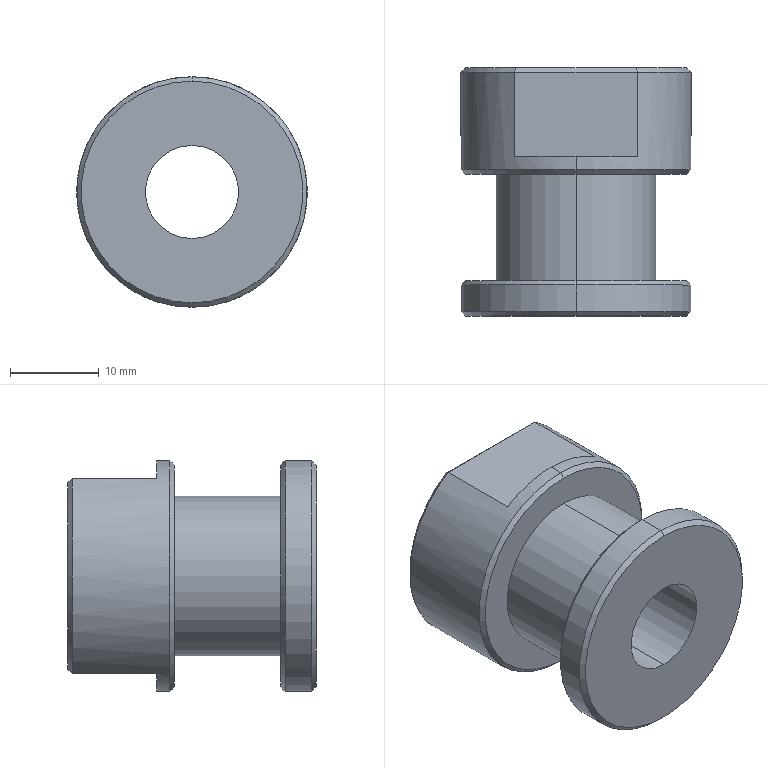Part | STEP file | 03-32SC Floating Joint | 1 solid | 52 faces | box 26 x 28 x 26 mm | volume 2635 mm3 | plane 20 | cone 16 | cylinder 16 | commonest cylinder face diameters 24.84 x4 26 x4 10.5 x2 12.16 x2 16.84 x2 18 x2
STEP:
#1=CARTESIAN_POINT('',(0.,-16.,-12.5));
#2=VERTEX_POINT('',#1);
#3=CARTESIAN_POINT('',(0.,-16.,12.5));
#4=VERTEX_POINT('',#3);
#5=CARTESIAN_POINT('',(0.,-16.,0.));
#6=DIRECTION('',(0.,-1.,0.));
#7=DIRECTION('',(0.,0.,-1.));
#8=AXIS2_PLACEMENT_3D('',#5,#6,#7);
#9=CIRCLE('',#8,12.5);
#10=EDGE_CURVE('',#2,#4,#9,.T.);
#11=ORIENTED_EDGE('',*,*,#10,.F.);
#12=CARTESIAN_POINT('',(0.,-15.5,-13.));
#13=VERTEX_POINT('',#12);
#14=CARTESIAN_POINT('',(0.,-16.,-12.5));
#15=DIRECTION('',(0.,0.7071,-0.7071));
#16=VECTOR('',#15,1000.);
#17=LINE('',#14,#16);
#18=EDGE_CURVE('',#2,#13,#17,.T.);
#19=ORIENTED_EDGE('',*,*,#18,.T.);
#20=CARTESIAN_POINT('',(0.,-15.5,13.));
#21=VERTEX_POINT('',#20);
#22=CARTESIAN_POINT('',(0.,-15.5,0.));
#23=DIRECTION('',(0.,1.,0.));
#24=DIRECTION('',(0.,0.,-1.));
#25=AXIS2_PLACEMENT_3D('',#22,#23,#24);
#26=CIRCLE('',#25,13.);
#27=EDGE_CURVE('',#21,#13,#26,.T.);
#28=ORIENTED_EDGE('',*,*,#27,.F.);
#29=CARTESIAN_POINT('',(0.,-16.,12.5));
#30=DIRECTION('',(0.,0.7071,0.7071));
#31=VECTOR('',#30,1000.);
#32=LINE('',#29,#31);
#33=EDGE_CURVE('',#4,#21,#32,.T.);
#34=ORIENTED_EDGE('',*,*,#33,.F.);
#35=EDGE_LOOP('',(#11,#19,#28,#34));
#36=FACE_OUTER_BOUND('',#35,.T.);
#37=CARTESIAN_POINT('',(0.,-16.,0.));
#38=DIRECTION('',(0.,1.,0.));
#39=DIRECTION('',(0.,0.,1.));
#40=AXIS2_PLACEMENT_3D('',#37,#38,#39);
#41=CONICAL_SURFACE('',#40,12.5,0.7854);
#42=ADVANCED_FACE('',(#36),#41,.T.);
#43=CARTESIAN_POINT('',(0.,0.,-12.5));
#44=VERTEX_POINT('',#43);
#45=CARTESIAN_POINT('',(0.,0.,12.5));
#46=VERTEX_POINT('',#45);
#47=CARTESIAN_POINT('',(0.,0.,0.));
#48=DIRECTION('',(0.,-1.,0.));
#49=DIRECTION('',(0.,0.,-1.));
#50=AXIS2_PLACEMENT_3D('',#47,#48,#49);
#51=CIRCLE('',#50,12.5);
#52=EDGE_CURVE('',#44,#46,#51,.T.);
#53=ORIENTED_EDGE('',*,*,#52,.F.);
#54=CARTESIAN_POINT('',(0.,0.5,-13.));
#55=VERTEX_POINT('',#54);
#56=CARTESIAN_POINT('',(0.,0.,-12.5));
#57=DIRECTION('',(0.,0.7071,-0.7071));
#58=VECTOR('',#57,1000.);
#59=LINE('',#56,#58);
#60=EDGE_CURVE('',#44,#55,#59,.T.);
#61=ORIENTED_EDGE('',*,*,#60,.T.);
#62=CARTESIAN_POINT('',(0.,0.5,13.));
#63=VERTEX_POINT('',#62);
#64=CARTESIAN_POINT('',(0.,0.5,0.));
#65=DIRECTION('',(0.,1.,0.));
#66=DIRECTION('',(0.,0.,-1.));
#67=AXIS2_PLACEMENT_3D('',#64,#65,#66);
#68=CIRCLE('',#67,13.);
#69=EDGE_CURVE('',#63,#55,#68,.T.);
#70=ORIENTED_EDGE('',*,*,#69,.F.);
#71=CARTESIAN_POINT('',(0.,0.,12.5));
#72=DIRECTION('',(0.,0.7071,0.7071));
#73=VECTOR('',#72,1000.);
#74=LINE('',#71,#73);
#75=EDGE_CURVE('',#46,#63,#74,.T.);
#76=ORIENTED_EDGE('',*,*,#75,.F.);
#77=EDGE_LOOP('',(#53,#61,#70,#76));
#78=FACE_OUTER_BOUND('',#77,.T.);
#79=CARTESIAN_POINT('',(0.,0.,0.));
#80=DIRECTION('',(0.,1.,0.));
#81=DIRECTION('',(0.,0.,1.));
#82=AXIS2_PLACEMENT_3D('',#79,#80,#81);
#83=CONICAL_SURFACE('',#82,12.5,0.7854);
#84=ADVANCED_FACE('',(#78),#83,.T.);
#85=CARTESIAN_POINT('',(0.,-12.,12.5));
#86=VERTEX_POINT('',#85);
#87=CARTESIAN_POINT('',(0.,-12.,-12.5));
#88=VERTEX_POINT('',#87);
#89=CARTESIAN_POINT('',(0.,-12.,0.));
#90=DIRECTION('',(0.,1.,0.));
#91=DIRECTION('',(0.,0.,1.));
#92=AXIS2_PLACEMENT_3D('',#89,#90,#91);
#93=CIRCLE('',#92,12.5);
#94=EDGE_CURVE('',#86,#88,#93,.T.);
#95=ORIENTED_EDGE('',*,*,#94,.F.);
#96=CARTESIAN_POINT('',(0.,-12.5,13.));
#97=VERTEX_POINT('',#96);
#98=CARTESIAN_POINT('',(0.,-12.5,13.));
#99=DIRECTION('',(0.,-0.7071,0.7071));
#100=VECTOR('',#99,1000.);
#101=LINE('',#98,#100);
#102=EDGE_CURVE('',#86,#97,#101,.T.);
#103=ORIENTED_EDGE('',*,*,#102,.T.);
#104=CARTESIAN_POINT('',(0.,-12.5,-13.));
#105=VERTEX_POINT('',#104);
#106=CARTESIAN_POINT('',(0.,-12.5,0.));
#107=DIRECTION('',(0.,-1.,0.));
#108=DIRECTION('',(0.,0.,1.));
#109=AXIS2_PLACEMENT_3D('',#106,#107,#108);
#110=CIRCLE('',#109,13.);
#111=EDGE_CURVE('',#105,#97,#110,.T.);
#112=ORIENTED_EDGE('',*,*,#111,.F.);
#113=CARTESIAN_POINT('',(0.,-12.5,-13.));
#114=DIRECTION('',(0.,-0.7071,-0.7071));
#115=VECTOR('',#114,1000.);
#116=LINE('',#113,#115);
#117=EDGE_CURVE('',#88,#105,#116,.T.);
#118=ORIENTED_EDGE('',*,*,#117,.F.);
#119=EDGE_LOOP('',(#95,#103,#112,#118));
#120=FACE_OUTER_BOUND('',#119,.T.);
#121=CARTESIAN_POINT('',(0.,-12.5,0.));
#122=DIRECTION('',(0.,-1.,0.));
#123=DIRECTION('',(0.,0.,-1.));
#124=AXIS2_PLACEMENT_3D('',#121,#122,#123);
#125=CONICAL_SURFACE('',#124,13.,0.7854);
#126=ADVANCED_FACE('',(#120),#125,.T.);
#127=CARTESIAN_POINT('',(0.,12.,-5.25));
#128=VERTEX_POINT('',#127);
#129=CARTESIAN_POINT('',(0.,12.,5.25));
#130=VERTEX_POINT('',#129);
#131=CARTESIAN_POINT('',(0.,12.,0.));
#132=DIRECTION('',(0.,1.,0.));
#133=DIRECTION('',(0.,0.,1.));
#134=AXIS2_PLACEMENT_3D('',#131,#132,#133);
#135=CIRCLE('',#134,5.25);
#136=EDGE_CURVE('',#128,#130,#135,.T.);
#137=ORIENTED_EDGE('',*,*,#136,.T.);
#138=CARTESIAN_POINT('',(0.,-16.,5.25));
#139=VERTEX_POINT('',#138);
#140=CARTESIAN_POINT('',(0.,-16.,5.25));
#141=DIRECTION('',(0.,-1.,0.));
#142=VECTOR('',#141,1000.);
#143=LINE('',#140,#142);
#144=EDGE_CURVE('',#130,#139,#143,.T.);
#145=ORIENTED_EDGE('',*,*,#144,.T.);
#146=CARTESIAN_POINT('',(0.,-16.,-5.25));
#147=VERTEX_POINT('',#146);
#148=CARTESIAN_POINT('',(0.,-16.,0.));
#149=DIRECTION('',(0.,-1.,0.));
#150=DIRECTION('',(0.,0.,-1.));
#151=AXIS2_PLACEMENT_3D('',#148,#149,#150);
#152=CIRCLE('',#151,5.25);
#153=EDGE_CURVE('',#139,#147,#152,.T.);
#154=ORIENTED_EDGE('',*,*,#153,.T.);
#155=CARTESIAN_POINT('',(0.,-16.,-5.25));
#156=DIRECTION('',(0.,-1.,0.));
#157=VECTOR('',#156,1000.);
#158=LINE('',#155,#157);
#159=EDGE_CURVE('',#128,#147,#158,.T.);
#160=ORIENTED_EDGE('',*,*,#159,.F.);
#161=EDGE_LOOP('',(#137,#145,#154,#160));
#162=FACE_OUTER_BOUND('',#161,.T.);
#163=CARTESIAN_POINT('',(0.,-16.,0.));
#164=DIRECTION('',(0.,-1.,0.));
#165=DIRECTION('',(0.,0.,-1.));
#166=AXIS2_PLACEMENT_3D('',#163,#164,#165);
#167=CYLINDRICAL_SURFACE('',#166,5.25);
#168=ADVANCED_FACE('',(#162),#167,.F.);
#169=CARTESIAN_POINT('',(0.,0.,-9.));
#170=VERTEX_POINT('',#169);
#171=CARTESIAN_POINT('',(0.,0.,9.));
#172=VERTEX_POINT('',#171);
#173=CARTESIAN_POINT('',(0.,0.,0.));
#174=DIRECTION('',(0.,-1.,0.));
#175=DIRECTION('',(0.,0.,-1.));
#176=AXIS2_PLACEMENT_3D('',#173,#174,#175);
#177=CIRCLE('',#176,9.);
#178=EDGE_CURVE('',#170,#172,#177,.T.);
#179=ORIENTED_EDGE('',*,*,#178,.T.);
#180=CARTESIAN_POINT('',(0.,-12.,9.));
#181=VERTEX_POINT('',#180);
#182=CARTESIAN_POINT('',(0.,12.,9.));
#183=DIRECTION('',(0.,-1.,0.));
#184=VECTOR('',#183,1000.);
#185=LINE('',#182,#184);
#186=EDGE_CURVE('',#172,#181,#185,.T.);
#187=ORIENTED_EDGE('',*,*,#186,.T.);
#188=CARTESIAN_POINT('',(0.,-12.,-9.));
#189=VERTEX_POINT('',#188);
#190=CARTESIAN_POINT('',(0.,-12.,0.));
#191=DIRECTION('',(0.,-1.,0.));
#192=DIRECTION('',(0.,0.,-1.));
#193=AXIS2_PLACEMENT_3D('',#190,#191,#192);
#194=CIRCLE('',#193,9.);
#195=EDGE_CURVE('',#189,#181,#194,.T.);
#196=ORIENTED_EDGE('',*,*,#195,.F.);
#197=CARTESIAN_POINT('',(0.,12.,-9.));
#198=DIRECTION('',(0.,-1.,0.));
#199=VECTOR('',#198,1000.);
#200=LINE('',#197,#199);
#201=EDGE_CURVE('',#170,#189,#200,.T.);
#202=ORIENTED_EDGE('',*,*,#201,.F.);
#203=EDGE_LOOP('',(#179,#187,#196,#202));
#204=FACE_OUTER_BOUND('',#203,.T.);
#205=CARTESIAN_POINT('',(0.,12.,0.));
#206=DIRECTION('',(0.,-1.,0.));
#207=DIRECTION('',(0.,0.,-1.));
#208=AXIS2_PLACEMENT_3D('',#205,#206,#207);
#209=CYLINDRICAL_SURFACE('',#208,9.);
#210=ADVANCED_FACE('',(#204),#209,.T.);
#211=ORIENTED_EDGE('',*,*,#111,.T.);
#212=CARTESIAN_POINT('',(0.,12.,13.));
#213=DIRECTION('',(0.,-1.,0.));
#214=VECTOR('',#213,1000.);
#215=LINE('',#212,#214);
#216=EDGE_CURVE('',#97,#21,#215,.T.);
#217=ORIENTED_EDGE('',*,*,#216,.T.);
#218=ORIENTED_EDGE('',*,*,#27,.T.);
#219=CARTESIAN_POINT('',(0.,12.,-13.));
#220=DIRECTION('',(0.,-1.,0.));
#221=VECTOR('',#220,1000.);
#222=LINE('',#219,#221);
#223=EDGE_CURVE('',#105,#13,#222,.T.);
#224=ORIENTED_EDGE('',*,*,#223,.F.);
#225=EDGE_LOOP('',(#211,#217,#218,#224));
#226=FACE_OUTER_BOUND('',#225,.T.);
#227=CARTESIAN_POINT('',(0.,12.,0.));
#228=DIRECTION('',(0.,-1.,0.));
#229=DIRECTION('',(0.,0.,-1.));
#230=AXIS2_PLACEMENT_3D('',#227,#228,#229);
#231=CYLINDRICAL_SURFACE('',#230,13.);
#232=ADVANCED_FACE('',(#226),#231,.T.);
#233=CARTESIAN_POINT('',(0.,2.,13.));
#234=VERTEX_POINT('',#233);
#235=CARTESIAN_POINT('',(6.928,2.,11.));
#236=VERTEX_POINT('',#235);
#237=CARTESIAN_POINT('',(0.,2.,0.));
#238=DIRECTION('',(0.,1.,0.));
#239=DIRECTION('',(0.,0.,1.));
#240=AXIS2_PLACEMENT_3D('',#237,#238,#239);
#241=CIRCLE('',#240,13.);
#242=EDGE_CURVE('',#234,#236,#241,.T.);
#243=ORIENTED_EDGE('',*,*,#242,.F.);
#244=CARTESIAN_POINT('',(0.,12.,13.));
#245=DIRECTION('',(0.,-1.,0.));
#246=VECTOR('',#245,1000.);
#247=LINE('',#244,#246);
#248=EDGE_CURVE('',#234,#63,#247,.T.);
#249=ORIENTED_EDGE('',*,*,#248,.T.);
#250=ORIENTED_EDGE('',*,*,#69,.T.);
#251=CARTESIAN_POINT('',(0.,2.,-13.));
#252=VERTEX_POINT('',#251);
#253=CARTESIAN_POINT('',(0.,12.,-13.));
#254=DIRECTION('',(0.,-1.,0.));
#255=VECTOR('',#254,1000.);
#256=LINE('',#253,#255);
#257=EDGE_CURVE('',#252,#55,#256,.T.);
#258=ORIENTED_EDGE('',*,*,#257,.F.);
#259=CARTESIAN_POINT('',(6.928,2.,-11.));
#260=VERTEX_POINT('',#259);
#261=CARTESIAN_POINT('',(0.,2.,0.));
#262=DIRECTION('',(0.,1.,0.));
#263=DIRECTION('',(0.,0.,1.));
#264=AXIS2_PLACEMENT_3D('',#261,#262,#263);
#265=CIRCLE('',#264,13.);
#266=EDGE_CURVE('',#260,#252,#265,.T.);
#267=ORIENTED_EDGE('',*,*,#266,.F.);
#268=CARTESIAN_POINT('',(6.928,11.5,-11.));
#269=VERTEX_POINT('',#268);
#270=CARTESIAN_POINT('',(6.928,2.,-11.));
#271=DIRECTION('',(0.,1.,0.));
#272=VECTOR('',#271,1000.);
#273=LINE('',#270,#272);
#274=EDGE_CURVE('',#260,#269,#273,.T.);
#275=ORIENTED_EDGE('',*,*,#274,.T.);
#276=CARTESIAN_POINT('',(6.928,11.5,11.));
#277=VERTEX_POINT('',#276);
#278=CARTESIAN_POINT('',(0.,11.5,0.));
#279=DIRECTION('',(0.,-1.,0.));
#280=DIRECTION('',(0.,0.,1.));
#281=AXIS2_PLACEMENT_3D('',#278,#279,#280);
#282=CIRCLE('',#281,13.);
#283=EDGE_CURVE('',#269,#277,#282,.T.);
#284=ORIENTED_EDGE('',*,*,#283,.T.);
#285=CARTESIAN_POINT('',(6.928,2.,11.));
#286=DIRECTION('',(0.,1.,0.));
#287=VECTOR('',#286,1000.);
#288=LINE('',#285,#287);
#289=EDGE_CURVE('',#236,#277,#288,.T.);
#290=ORIENTED_EDGE('',*,*,#289,.F.);
#291=EDGE_LOOP('',(#243,#249,#250,#258,#267,#275,#284,#290));
#292=FACE_OUTER_BOUND('',#291,.T.);
#293=CARTESIAN_POINT('',(0.,12.,0.));
#294=DIRECTION('',(0.,-1.,0.));
#295=DIRECTION('',(0.,0.,-1.));
#296=AXIS2_PLACEMENT_3D('',#293,#294,#295);
#297=CYLINDRICAL_SURFACE('',#296,13.);
#298=ADVANCED_FACE('',(#292),#297,.T.);
#299=ORIENTED_EDGE('',*,*,#248,.F.);
#300=CARTESIAN_POINT('',(-6.928,2.,11.));
#301=VERTEX_POINT('',#300);
#302=CARTESIAN_POINT('',(0.,2.,0.));
#303=DIRECTION('',(0.,1.,0.));
#304=DIRECTION('',(0.,0.,1.));
#305=AXIS2_PLACEMENT_3D('',#302,#303,#304);
#306=CIRCLE('',#305,13.);
#307=EDGE_CURVE('',#301,#234,#306,.T.);
#308=ORIENTED_EDGE('',*,*,#307,.F.);
#309=CARTESIAN_POINT('',(-6.928,11.5,11.));
#310=VERTEX_POINT('',#309);
#311=CARTESIAN_POINT('',(-6.928,2.,11.));
#312=DIRECTION('',(0.,1.,0.));
#313=VECTOR('',#312,1000.);
#314=LINE('',#311,#313);
#315=EDGE_CURVE('',#301,#310,#314,.T.);
#316=ORIENTED_EDGE('',*,*,#315,.T.);
#317=CARTESIAN_POINT('',(-6.928,11.5,-11.));
#318=VERTEX_POINT('',#317);
#319=CARTESIAN_POINT('',(0.,11.5,0.));
#320=DIRECTION('',(0.,-1.,0.));
#321=DIRECTION('',(0.,0.,1.));
#322=AXIS2_PLACEMENT_3D('',#319,#320,#321);
#323=CIRCLE('',#322,13.);
#324=EDGE_CURVE('',#310,#318,#323,.T.);
#325=ORIENTED_EDGE('',*,*,#324,.T.);
#326=CARTESIAN_POINT('',(-6.928,2.,-11.));
#327=VERTEX_POINT('',#326);
#328=CARTESIAN_POINT('',(-6.928,2.,-11.));
#329=DIRECTION('',(0.,1.,0.));
#330=VECTOR('',#329,1000.);
#331=LINE('',#328,#330);
#332=EDGE_CURVE('',#327,#318,#331,.T.);
#333=ORIENTED_EDGE('',*,*,#332,.F.);
#334=CARTESIAN_POINT('',(0.,2.,0.));
#335=DIRECTION('',(0.,1.,0.));
#336=DIRECTION('',(0.,0.,1.));
#337=AXIS2_PLACEMENT_3D('',#334,#335,#336);
#338=CIRCLE('',#337,13.);
#339=EDGE_CURVE('',#252,#327,#338,.T.);
#340=ORIENTED_EDGE('',*,*,#339,.F.);
#341=ORIENTED_EDGE('',*,*,#257,.T.);
#342=CARTESIAN_POINT('',(0.,0.5,0.));
#343=DIRECTION('',(0.,1.,0.));
#344=DIRECTION('',(0.,0.,-1.));
#345=AXIS2_PLACEMENT_3D('',#342,#343,#344);
#346=CIRCLE('',#345,13.);
#347=EDGE_CURVE('',#55,#63,#346,.T.);
#348=ORIENTED_EDGE('',*,*,#347,.T.);
#349=EDGE_LOOP('',(#299,#308,#316,#325,#333,#340,#341,#348));
#350=FACE_OUTER_BOUND('',#349,.T.);
#351=CARTESIAN_POINT('',(0.,12.,0.));
#352=DIRECTION('',(0.,-1.,0.));
#353=DIRECTION('',(0.,0.,-1.));
#354=AXIS2_PLACEMENT_3D('',#351,#352,#353);
#355=CYLINDRICAL_SURFACE('',#354,13.);
#356=ADVANCED_FACE('',(#350),#355,.T.);
#357=CARTESIAN_POINT('',(-6.782,12.,10.5));
#358=VERTEX_POINT('',#357);
#359=CARTESIAN_POINT('',(6.782,12.,10.5));
#360=VERTEX_POINT('',#359);
#361=CARTESIAN_POINT('',(6.928,12.,10.5));
#362=DIRECTION('',(1.,0.,0.));
#363=VECTOR('',#362,1000.);
#364=LINE('',#361,#363);
#365=EDGE_CURVE('',#358,#360,#364,.T.);
#366=ORIENTED_EDGE('',*,*,#365,.T.);
#367=CARTESIAN_POINT('',(6.782,12.,-10.5));
#368=VERTEX_POINT('',#367);
#369=CARTESIAN_POINT('',(0.,12.,0.));
#370=DIRECTION('',(0.,1.,0.));
#371=DIRECTION('',(0.,0.,1.));
#372=AXIS2_PLACEMENT_3D('',#369,#370,#371);
#373=CIRCLE('',#372,12.5);
#374=EDGE_CURVE('',#360,#368,#373,.T.);
#375=ORIENTED_EDGE('',*,*,#374,.T.);
#376=CARTESIAN_POINT('',(-6.782,12.,-10.5));
#377=VERTEX_POINT('',#376);
#378=CARTESIAN_POINT('',(-6.928,12.,-10.5));
#379=DIRECTION('',(-1.,0.,0.));
#380=VECTOR('',#379,1000.);
#381=LINE('',#378,#380);
#382=EDGE_CURVE('',#368,#377,#381,.T.);
#383=ORIENTED_EDGE('',*,*,#382,.T.);
#384=CARTESIAN_POINT('',(0.,12.,0.));
#385=DIRECTION('',(0.,1.,0.));
#386=DIRECTION('',(0.,0.,1.));
#387=AXIS2_PLACEMENT_3D('',#384,#385,#386);
#388=CIRCLE('',#387,12.5);
#389=EDGE_CURVE('',#377,#358,#388,.T.);
#390=ORIENTED_EDGE('',*,*,#389,.T.);
#391=EDGE_LOOP('',(#366,#375,#383,#390));
#392=FACE_OUTER_BOUND('',#391,.T.);
#393=ORIENTED_EDGE('',*,*,#136,.F.);
#394=CARTESIAN_POINT('',(0.,12.,0.));
#395=DIRECTION('',(0.,1.,0.));
#396=DIRECTION('',(0.,0.,1.));
#397=AXIS2_PLACEMENT_3D('',#394,#395,#396);
#398=CIRCLE('',#397,5.25);
#399=EDGE_CURVE('',#130,#128,#398,.T.);
#400=ORIENTED_EDGE('',*,*,#399,.F.);
#401=EDGE_LOOP('',(#393,#400));
#402=FACE_BOUND('',#401,.T.);
#403=CARTESIAN_POINT('',(13.,12.,0.));
#404=DIRECTION('',(0.,1.,0.));
#405=DIRECTION('',(0.,0.,1.));
#406=AXIS2_PLACEMENT_3D('',#403,#404,#405);
#407=PLANE('',#406);
#408=ADVANCED_FACE('',(#392,#402),#407,.T.);
#409=CARTESIAN_POINT('',(0.,-16.,0.));
#410=DIRECTION('',(0.,-1.,0.));
#411=DIRECTION('',(0.,0.,-1.));
#412=AXIS2_PLACEMENT_3D('',#409,#410,#411);
#413=CIRCLE('',#412,12.5);
#414=EDGE_CURVE('',#4,#2,#413,.T.);
#415=ORIENTED_EDGE('',*,*,#414,.T.);
#416=ORIENTED_EDGE('',*,*,#10,.T.);
#417=EDGE_LOOP('',(#415,#416));
#418=FACE_OUTER_BOUND('',#417,.T.);
#419=CARTESIAN_POINT('',(0.,-16.,0.));
#420=DIRECTION('',(0.,-1.,0.));
#421=DIRECTION('',(0.,0.,-1.));
#422=AXIS2_PLACEMENT_3D('',#419,#420,#421);
#423=CIRCLE('',#422,5.25);
#424=EDGE_CURVE('',#147,#139,#423,.T.);
#425=ORIENTED_EDGE('',*,*,#424,.F.);
#426=ORIENTED_EDGE('',*,*,#153,.F.);
#427=EDGE_LOOP('',(#425,#426));
#428=FACE_BOUND('',#427,.T.);
#429=CARTESIAN_POINT('',(0.,-16.,0.));
#430=DIRECTION('',(0.,-1.,0.));
#431=DIRECTION('',(0.,0.,-1.));
#432=AXIS2_PLACEMENT_3D('',#429,#430,#431);
#433=PLANE('',#432);
#434=ADVANCED_FACE('',(#418,#428),#433,.T.);
#435=ORIENTED_EDGE('',*,*,#216,.F.);
#436=CARTESIAN_POINT('',(0.,-12.5,0.));
#437=DIRECTION('',(0.,-1.,0.));
#438=DIRECTION('',(0.,0.,1.));
#439=AXIS2_PLACEMENT_3D('',#436,#437,#438);
#440=CIRCLE('',#439,13.);
#441=EDGE_CURVE('',#97,#105,#440,.T.);
#442=ORIENTED_EDGE('',*,*,#441,.T.);
#443=ORIENTED_EDGE('',*,*,#223,.T.);
#444=CARTESIAN_POINT('',(0.,-15.5,0.));
#445=DIRECTION('',(0.,1.,0.));
#446=DIRECTION('',(0.,0.,-1.));
#447=AXIS2_PLACEMENT_3D('',#444,#445,#446);
#448=CIRCLE('',#447,13.);
#449=EDGE_CURVE('',#13,#21,#448,.T.);
#450=ORIENTED_EDGE('',*,*,#449,.T.);
#451=EDGE_LOOP('',(#435,#442,#443,#450));
#452=FACE_OUTER_BOUND('',#451,.T.);
#453=CARTESIAN_POINT('',(0.,12.,0.));
#454=DIRECTION('',(0.,-1.,0.));
#455=DIRECTION('',(0.,0.,-1.));
#456=AXIS2_PLACEMENT_3D('',#453,#454,#455);
#457=CYLINDRICAL_SURFACE('',#456,13.);
#458=ADVANCED_FACE('',(#452),#457,.T.);
#459=CARTESIAN_POINT('',(0.,-12.,0.));
#460=DIRECTION('',(0.,1.,0.));
#461=DIRECTION('',(0.,0.,1.));
#462=AXIS2_PLACEMENT_3D('',#459,#460,#461);
#463=CIRCLE('',#462,12.5);
#464=EDGE_CURVE('',#88,#86,#463,.T.);
#465=ORIENTED_EDGE('',*,*,#464,.T.);
#466=ORIENTED_EDGE('',*,*,#94,.T.);
#467=EDGE_LOOP('',(#465,#466));
#468=FACE_OUTER_BOUND('',#467,.T.);
#469=ORIENTED_EDGE('',*,*,#195,.T.);
#470=CARTESIAN_POINT('',(0.,-12.,0.));
#471=DIRECTION('',(0.,-1.,0.));
#472=DIRECTION('',(0.,0.,-1.));
#473=AXIS2_PLACEMENT_3D('',#470,#471,#472);
#474=CIRCLE('',#473,9.);
#475=EDGE_CURVE('',#181,#189,#474,.T.);
#476=ORIENTED_EDGE('',*,*,#475,.T.);
#477=EDGE_LOOP('',(#469,#476));
#478=FACE_BOUND('',#477,.T.);
#479=CARTESIAN_POINT('',(13.,-12.,0.));
#480=DIRECTION('',(0.,1.,0.));
#481=DIRECTION('',(0.,0.,1.));
#482=AXIS2_PLACEMENT_3D('',#479,#480,#481);
#483=PLANE('',#482);
#484=ADVANCED_FACE('',(#468,#478),#483,.T.);
#485=ORIENTED_EDGE('',*,*,#186,.F.);
#486=CARTESIAN_POINT('',(0.,0.,0.));
#487=DIRECTION('',(0.,-1.,0.));
#488=DIRECTION('',(0.,0.,-1.));
#489=AXIS2_PLACEMENT_3D('',#486,#487,#488);
#490=CIRCLE('',#489,9.);
#491=EDGE_CURVE('',#172,#170,#490,.T.);
#492=ORIENTED_EDGE('',*,*,#491,.T.);
#493=ORIENTED_EDGE('',*,*,#201,.T.);
#494=ORIENTED_EDGE('',*,*,#475,.F.);
#495=EDGE_LOOP('',(#485,#492,#493,#494));
#496=FACE_OUTER_BOUND('',#495,.T.);
#497=CARTESIAN_POINT('',(0.,12.,0.));
#498=DIRECTION('',(0.,-1.,0.));
#499=DIRECTION('',(0.,0.,-1.));
#500=AXIS2_PLACEMENT_3D('',#497,#498,#499);
#501=CYLINDRICAL_SURFACE('',#500,9.);
#502=ADVANCED_FACE('',(#496),#501,.T.);
#503=CARTESIAN_POINT('',(0.,0.,0.));
#504=DIRECTION('',(0.,-1.,0.));
#505=DIRECTION('',(0.,0.,-1.));
#506=AXIS2_PLACEMENT_3D('',#503,#504,#505);
#507=CIRCLE('',#506,12.5);
#508=EDGE_CURVE('',#46,#44,#507,.T.);
#509=ORIENTED_EDGE('',*,*,#508,.T.);
#510=ORIENTED_EDGE('',*,*,#52,.T.);
#511=EDGE_LOOP('',(#509,#510));
#512=FACE_OUTER_BOUND('',#511,.T.);
#513=ORIENTED_EDGE('',*,*,#178,.F.);
#514=ORIENTED_EDGE('',*,*,#491,.F.);
#515=EDGE_LOOP('',(#513,#514));
#516=FACE_BOUND('',#515,.T.);
#517=CARTESIAN_POINT('',(9.,0.,0.));
#518=DIRECTION('',(0.,-1.,0.));
#519=DIRECTION('',(0.,0.,-1.));
#520=AXIS2_PLACEMENT_3D('',#517,#518,#519);
#521=PLANE('',#520);
#522=ADVANCED_FACE('',(#512,#516),#521,.T.);
#523=ORIENTED_EDGE('',*,*,#332,.T.);
#524=CARTESIAN_POINT('',(6.928,11.5,-11.));
#525=DIRECTION('',(1.,0.,0.));
#526=VECTOR('',#525,1000.);
#527=LINE('',#524,#526);
#528=EDGE_CURVE('',#318,#269,#527,.T.);
#529=ORIENTED_EDGE('',*,*,#528,.T.);
#530=ORIENTED_EDGE('',*,*,#274,.F.);
#531=CARTESIAN_POINT('',(-6.928,2.,-11.));
#532=DIRECTION('',(1.,0.,0.));
#533=VECTOR('',#532,1000.);
#534=LINE('',#531,#533);
#535=EDGE_CURVE('',#327,#260,#534,.T.);
#536=ORIENTED_EDGE('',*,*,#535,.F.);
#537=EDGE_LOOP('',(#523,#529,#530,#536));
#538=FACE_OUTER_BOUND('',#537,.T.);
#539=CARTESIAN_POINT('',(-6.928,2.,-11.));
#540=DIRECTION('',(0.,0.,1.));
#541=DIRECTION('',(1.,0.,0.));
#542=AXIS2_PLACEMENT_3D('',#539,#540,#541);
#543=PLANE('',#542);
#544=ADVANCED_FACE('',(#538),#543,.F.);
#545=ORIENTED_EDGE('',*,*,#266,.T.);
#546=ORIENTED_EDGE('',*,*,#339,.T.);
#547=ORIENTED_EDGE('',*,*,#535,.T.);
#548=EDGE_LOOP('',(#545,#546,#547));
#549=FACE_OUTER_BOUND('',#548,.T.);
#550=CARTESIAN_POINT('',(0.,2.,0.));
#551=DIRECTION('',(0.,1.,0.));
#552=DIRECTION('',(0.,0.,1.));
#553=AXIS2_PLACEMENT_3D('',#550,#551,#552);
#554=PLANE('',#553);
#555=ADVANCED_FACE('',(#549),#554,.T.);
#556=ORIENTED_EDGE('',*,*,#289,.T.);
#557=CARTESIAN_POINT('',(-6.928,11.5,11.));
#558=DIRECTION('',(-1.,0.,0.));
#559=VECTOR('',#558,1000.);
#560=LINE('',#557,#559);
#561=EDGE_CURVE('',#277,#310,#560,.T.);
#562=ORIENTED_EDGE('',*,*,#561,.T.);
#563=ORIENTED_EDGE('',*,*,#315,.F.);
#564=CARTESIAN_POINT('',(6.928,2.,11.));
#565=DIRECTION('',(-1.,0.,0.));
#566=VECTOR('',#565,1000.);
#567=LINE('',#564,#566);
#568=EDGE_CURVE('',#236,#301,#567,.T.);
#569=ORIENTED_EDGE('',*,*,#568,.F.);
#570=EDGE_LOOP('',(#556,#562,#563,#569));
#571=FACE_OUTER_BOUND('',#570,.T.);
#572=CARTESIAN_POINT('',(6.928,2.,11.));
#573=DIRECTION('',(0.,0.,-1.));
#574=DIRECTION('',(-1.,0.,0.));
#575=AXIS2_PLACEMENT_3D('',#572,#573,#574);
#576=PLANE('',#575);
#577=ADVANCED_FACE('',(#571),#576,.F.);
#578=ORIENTED_EDGE('',*,*,#307,.T.);
#579=ORIENTED_EDGE('',*,*,#242,.T.);
#580=ORIENTED_EDGE('',*,*,#568,.T.);
#581=EDGE_LOOP('',(#578,#579,#580));
#582=FACE_OUTER_BOUND('',#581,.T.);
#583=CARTESIAN_POINT('',(0.,2.,0.));
#584=DIRECTION('',(0.,1.,0.));
#585=DIRECTION('',(0.,0.,1.));
#586=AXIS2_PLACEMENT_3D('',#583,#584,#585);
#587=PLANE('',#586);
#588=ADVANCED_FACE('',(#582),#587,.T.);
#589=ORIENTED_EDGE('',*,*,#144,.F.);
#590=ORIENTED_EDGE('',*,*,#399,.T.);
#591=ORIENTED_EDGE('',*,*,#159,.T.);
#592=ORIENTED_EDGE('',*,*,#424,.T.);
#593=EDGE_LOOP('',(#589,#590,#591,#592));
#594=FACE_OUTER_BOUND('',#593,.T.);
#595=CARTESIAN_POINT('',(0.,-16.,0.));
#596=DIRECTION('',(0.,-1.,0.));
#597=DIRECTION('',(0.,0.,-1.));
#598=AXIS2_PLACEMENT_3D('',#595,#596,#597);
#599=CYLINDRICAL_SURFACE('',#598,5.25);
#600=ADVANCED_FACE('',(#594),#599,.F.);
#601=ORIENTED_EDGE('',*,*,#102,.F.);
#602=ORIENTED_EDGE('',*,*,#464,.F.);
#603=ORIENTED_EDGE('',*,*,#117,.T.);
#604=ORIENTED_EDGE('',*,*,#441,.F.);
#605=EDGE_LOOP('',(#601,#602,#603,#604));
#606=FACE_OUTER_BOUND('',#605,.T.);
#607=CARTESIAN_POINT('',(0.,-12.5,0.));
#608=DIRECTION('',(0.,-1.,0.));
#609=DIRECTION('',(0.,0.,-1.));
#610=AXIS2_PLACEMENT_3D('',#607,#608,#609);
#611=CONICAL_SURFACE('',#610,13.,0.7854);
#612=ADVANCED_FACE('',(#606),#611,.T.);
#613=CARTESIAN_POINT('',(-6.782,12.,10.5));
#614=CARTESIAN_POINT('',(-6.831,11.833,10.667));
#615=CARTESIAN_POINT('',(-6.88,11.667,10.833));
#616=CARTESIAN_POINT('',(-6.928,11.5,11.));
#617=B_SPLINE_CURVE_WITH_KNOTS('',3,(#613,#614,#615,#616),.UNSPECIFIED.,.F.,.F.,(4,4),(0.,0.000722),.UNSPECIFIED.);
#618=EDGE_CURVE('',#358,#310,#617,.T.);
#619=ORIENTED_EDGE('',*,*,#618,.F.);
#620=ORIENTED_EDGE('',*,*,#389,.F.);
#621=CARTESIAN_POINT('',(-6.928,11.5,-11.));
#622=CARTESIAN_POINT('',(-6.88,11.667,-10.833));
#623=CARTESIAN_POINT('',(-6.831,11.833,-10.667));
#624=CARTESIAN_POINT('',(-6.782,12.,-10.5));
#625=B_SPLINE_CURVE_WITH_KNOTS('',3,(#621,#622,#623,#624),.UNSPECIFIED.,.F.,.F.,(4,4),(0.,0.000722),.UNSPECIFIED.);
#626=EDGE_CURVE('',#318,#377,#625,.T.);
#627=ORIENTED_EDGE('',*,*,#626,.F.);
#628=ORIENTED_EDGE('',*,*,#324,.F.);
#629=EDGE_LOOP('',(#619,#620,#627,#628));
#630=FACE_OUTER_BOUND('',#629,.T.);
#631=CARTESIAN_POINT('',(0.,11.5,0.));
#632=DIRECTION('',(0.,-1.,0.));
#633=DIRECTION('',(0.,0.,-1.));
#634=AXIS2_PLACEMENT_3D('',#631,#632,#633);
#635=CONICAL_SURFACE('',#634,13.,0.7854);
#636=ADVANCED_FACE('',(#630),#635,.T.);
#637=ORIENTED_EDGE('',*,*,#626,.T.);
#638=ORIENTED_EDGE('',*,*,#382,.F.);
#639=CARTESIAN_POINT('',(6.928,11.5,-11.));
#640=CARTESIAN_POINT('',(6.88,11.667,-10.833));
#641=CARTESIAN_POINT('',(6.831,11.833,-10.667));
#642=CARTESIAN_POINT('',(6.782,12.,-10.5));
#643=B_SPLINE_CURVE_WITH_KNOTS('',3,(#639,#640,#641,#642),.UNSPECIFIED.,.F.,.F.,(4,4),(0.,0.000722),.UNSPECIFIED.);
#644=EDGE_CURVE('',#269,#368,#643,.T.);
#645=ORIENTED_EDGE('',*,*,#644,.F.);
#646=ORIENTED_EDGE('',*,*,#528,.F.);
#647=EDGE_LOOP('',(#637,#638,#645,#646));
#648=FACE_OUTER_BOUND('',#647,.T.);
#649=CARTESIAN_POINT('',(-6.928,11.5,-11.));
#650=DIRECTION('',(0.,0.7071,-0.7071));
#651=DIRECTION('',(0.,0.7071,0.7071));
#652=AXIS2_PLACEMENT_3D('',#649,#650,#651);
#653=PLANE('',#652);
#654=ADVANCED_FACE('',(#648),#653,.T.);
#655=ORIENTED_EDGE('',*,*,#618,.T.);
#656=ORIENTED_EDGE('',*,*,#561,.F.);
#657=CARTESIAN_POINT('',(6.782,12.,10.5));
#658=CARTESIAN_POINT('',(6.831,11.833,10.667));
#659=CARTESIAN_POINT('',(6.88,11.667,10.833));
#660=CARTESIAN_POINT('',(6.928,11.5,11.));
#661=B_SPLINE_CURVE_WITH_KNOTS('',3,(#657,#658,#659,#660),.UNSPECIFIED.,.F.,.F.,(4,4),(0.,0.000722),.UNSPECIFIED.);
#662=EDGE_CURVE('',#360,#277,#661,.T.);
#663=ORIENTED_EDGE('',*,*,#662,.F.);
#664=ORIENTED_EDGE('',*,*,#365,.F.);
#665=EDGE_LOOP('',(#655,#656,#663,#664));
#666=FACE_OUTER_BOUND('',#665,.T.);
#667=CARTESIAN_POINT('',(6.928,11.5,11.));
#668=DIRECTION('',(0.,0.7071,0.7071));
#669=DIRECTION('',(0.,-0.7071,0.7071));
#670=AXIS2_PLACEMENT_3D('',#667,#668,#669);
#671=PLANE('',#670);
#672=ADVANCED_FACE('',(#666),#671,.T.);
#673=ORIENTED_EDGE('',*,*,#644,.T.);
#674=ORIENTED_EDGE('',*,*,#374,.F.);
#675=ORIENTED_EDGE('',*,*,#662,.T.);
#676=ORIENTED_EDGE('',*,*,#283,.F.);
#677=EDGE_LOOP('',(#673,#674,#675,#676));
#678=FACE_OUTER_BOUND('',#677,.T.);
#679=CARTESIAN_POINT('',(0.,11.5,0.));
#680=DIRECTION('',(0.,-1.,0.));
#681=DIRECTION('',(0.,0.,-1.));
#682=AXIS2_PLACEMENT_3D('',#679,#680,#681);
#683=CONICAL_SURFACE('',#682,13.,0.7854);
#684=ADVANCED_FACE('',(#678),#683,.T.);
#685=ORIENTED_EDGE('',*,*,#60,.F.);
#686=ORIENTED_EDGE('',*,*,#508,.F.);
#687=ORIENTED_EDGE('',*,*,#75,.T.);
#688=ORIENTED_EDGE('',*,*,#347,.F.);
#689=EDGE_LOOP('',(#685,#686,#687,#688));
#690=FACE_OUTER_BOUND('',#689,.T.);
#691=CARTESIAN_POINT('',(0.,0.,0.));
#692=DIRECTION('',(0.,1.,0.));
#693=DIRECTION('',(0.,0.,1.));
#694=AXIS2_PLACEMENT_3D('',#691,#692,#693);
#695=CONICAL_SURFACE('',#694,12.5,0.7854);
#696=ADVANCED_FACE('',(#690),#695,.T.);
#697=ORIENTED_EDGE('',*,*,#18,.F.);
#698=ORIENTED_EDGE('',*,*,#414,.F.);
#699=ORIENTED_EDGE('',*,*,#33,.T.);
#700=ORIENTED_EDGE('',*,*,#449,.F.);
#701=EDGE_LOOP('',(#697,#698,#699,#700));
#702=FACE_OUTER_BOUND('',#701,.T.);
#703=CARTESIAN_POINT('',(0.,-16.,0.));
#704=DIRECTION('',(0.,1.,0.));
#705=DIRECTION('',(0.,0.,1.));
#706=AXIS2_PLACEMENT_3D('',#703,#704,#705);
#707=CONICAL_SURFACE('',#706,12.5,0.7854);
#708=ADVANCED_FACE('',(#702),#707,.T.);
#709=CLOSED_SHELL('',(#42,#84,#126,#168,#210,#232,#298,#356,#408,#434,#458,#484,#502,#522,#544,#555,#577,#588,#600,#612,#636,#654,#672,#684,#696,#708));
#710=CARTESIAN_POINT('',(0.,-12.58,12.26));
#711=VERTEX_POINT('',#710);
#712=CARTESIAN_POINT('',(0.,-12.58,-12.26));
#713=VERTEX_POINT('',#712);
#714=CARTESIAN_POINT('',(0.,-12.58,0.));
#715=DIRECTION('',(0.,-1.,0.));
#716=DIRECTION('',(0.,0.,-1.));
#717=AXIS2_PLACEMENT_3D('',#714,#715,#716);
#718=CIRCLE('',#717,12.26);
#719=EDGE_CURVE('',#711,#713,#718,.T.);
#720=ORIENTED_EDGE('',*,*,#719,.F.);
#721=CARTESIAN_POINT('',(0.,-12.74,12.42));
#722=VERTEX_POINT('',#721);
#723=CARTESIAN_POINT('',(0.,-12.74,12.42));
#724=DIRECTION('',(0.,-0.7071,0.7071));
#725=VECTOR('',#724,1000.);
#726=LINE('',#723,#725);
#727=EDGE_CURVE('',#711,#722,#726,.T.);
#728=ORIENTED_EDGE('',*,*,#727,.T.);
#729=CARTESIAN_POINT('',(0.,-12.74,-12.42));
#730=VERTEX_POINT('',#729);
#731=CARTESIAN_POINT('',(0.,-12.74,0.));
#732=DIRECTION('',(0.,1.,0.));
#733=DIRECTION('',(0.,0.,-1.));
#734=AXIS2_PLACEMENT_3D('',#731,#732,#733);
#735=CIRCLE('',#734,12.42);
#736=EDGE_CURVE('',#730,#722,#735,.T.);
#737=ORIENTED_EDGE('',*,*,#736,.F.);
#738=CARTESIAN_POINT('',(0.,-12.74,-12.42));
#739=DIRECTION('',(0.,-0.7071,-0.7071));
#740=VECTOR('',#739,1000.);
#741=LINE('',#738,#740);
#742=EDGE_CURVE('',#713,#730,#741,.T.);
#743=ORIENTED_EDGE('',*,*,#742,.F.);
#744=EDGE_LOOP('',(#720,#728,#737,#743));
#745=FACE_OUTER_BOUND('',#744,.T.);
#746=CARTESIAN_POINT('',(0.,-12.74,0.));
#747=DIRECTION('',(0.,-1.,0.));
#748=DIRECTION('',(0.,0.,-1.));
#749=AXIS2_PLACEMENT_3D('',#746,#747,#748);
#750=CONICAL_SURFACE('',#749,12.42,0.7854);
#751=ADVANCED_FACE('',(#745),#750,.F.);
#752=CARTESIAN_POINT('',(0.,0.58,-12.26));
#753=VERTEX_POINT('',#752);
#754=CARTESIAN_POINT('',(0.,0.58,12.26));
#755=VERTEX_POINT('',#754);
#756=CARTESIAN_POINT('',(0.,0.58,0.));
#757=DIRECTION('',(0.,1.,0.));
#758=DIRECTION('',(0.,0.,-1.));
#759=AXIS2_PLACEMENT_3D('',#756,#757,#758);
#760=CIRCLE('',#759,12.26);
#761=EDGE_CURVE('',#753,#755,#760,.T.);
#762=ORIENTED_EDGE('',*,*,#761,.F.);
#763=CARTESIAN_POINT('',(0.,0.7402,-12.42));
#764=VERTEX_POINT('',#763);
#765=CARTESIAN_POINT('',(0.,0.58,-12.26));
#766=DIRECTION('',(0.,0.7071,-0.7071));
#767=VECTOR('',#766,1000.);
#768=LINE('',#765,#767);
#769=EDGE_CURVE('',#753,#764,#768,.T.);
#770=ORIENTED_EDGE('',*,*,#769,.T.);
#771=CARTESIAN_POINT('',(0.,0.7402,12.42));
#772=VERTEX_POINT('',#771);
#773=CARTESIAN_POINT('',(0.,0.7402,0.));
#774=DIRECTION('',(0.,-1.,0.));
#775=DIRECTION('',(0.,0.,-1.));
#776=AXIS2_PLACEMENT_3D('',#773,#774,#775);
#777=CIRCLE('',#776,12.42);
#778=EDGE_CURVE('',#772,#764,#777,.T.);
#779=ORIENTED_EDGE('',*,*,#778,.F.);
#780=CARTESIAN_POINT('',(0.,0.58,12.26));
#781=DIRECTION('',(0.,0.7071,0.7071));
#782=VECTOR('',#781,1000.);
#783=LINE('',#780,#782);
#784=EDGE_CURVE('',#755,#772,#783,.T.);
#785=ORIENTED_EDGE('',*,*,#784,.F.);
#786=EDGE_LOOP('',(#762,#770,#779,#785));
#787=FACE_OUTER_BOUND('',#786,.T.);
#788=CARTESIAN_POINT('',(0.,0.58,0.));
#789=DIRECTION('',(0.,1.,0.));
#790=DIRECTION('',(0.,0.,1.));
#791=AXIS2_PLACEMENT_3D('',#788,#789,#790);
#792=CONICAL_SURFACE('',#791,12.26,0.7854);
#793=ADVANCED_FACE('',(#787),#792,.F.);
#794=CARTESIAN_POINT('',(0.,-15.42,-12.26));
#795=VERTEX_POINT('',#794);
#796=CARTESIAN_POINT('',(0.,-15.42,12.26));
#797=VERTEX_POINT('',#796);
#798=CARTESIAN_POINT('',(0.,-15.42,0.));
#799=DIRECTION('',(0.,1.,0.));
#800=DIRECTION('',(0.,0.,-1.));
#801=AXIS2_PLACEMENT_3D('',#798,#799,#800);
#802=CIRCLE('',#801,12.26);
#803=EDGE_CURVE('',#795,#797,#802,.T.);
#804=ORIENTED_EDGE('',*,*,#803,.F.);
#805=CARTESIAN_POINT('',(0.,-15.26,-12.42));
#806=VERTEX_POINT('',#805);
#807=CARTESIAN_POINT('',(0.,-15.42,-12.26));
#808=DIRECTION('',(0.,0.7071,-0.7071));
#809=VECTOR('',#808,1000.);
#810=LINE('',#807,#809);
#811=EDGE_CURVE('',#795,#806,#810,.T.);
#812=ORIENTED_EDGE('',*,*,#811,.T.);
#813=CARTESIAN_POINT('',(0.,-15.26,12.42));
#814=VERTEX_POINT('',#813);
#815=CARTESIAN_POINT('',(0.,-15.26,0.));
#816=DIRECTION('',(0.,-1.,0.));
#817=DIRECTION('',(0.,0.,-1.));
#818=AXIS2_PLACEMENT_3D('',#815,#816,#817);
#819=CIRCLE('',#818,12.42);
#820=EDGE_CURVE('',#814,#806,#819,.T.);
#821=ORIENTED_EDGE('',*,*,#820,.F.);
#822=CARTESIAN_POINT('',(0.,-15.42,12.26));
#823=DIRECTION('',(0.,0.7071,0.7071));
#824=VECTOR('',#823,1000.);
#825=LINE('',#822,#824);
#826=EDGE_CURVE('',#797,#814,#825,.T.);
#827=ORIENTED_EDGE('',*,*,#826,.F.);
#828=EDGE_LOOP('',(#804,#812,#821,#827));
#829=FACE_OUTER_BOUND('',#828,.T.);
#830=CARTESIAN_POINT('',(0.,-15.42,0.));
#831=DIRECTION('',(0.,1.,0.));
#832=DIRECTION('',(0.,0.,1.));
#833=AXIS2_PLACEMENT_3D('',#830,#831,#832);
#834=CONICAL_SURFACE('',#833,12.26,0.7854);
#835=ADVANCED_FACE('',(#829),#834,.F.);
#836=CARTESIAN_POINT('',(0.,-15.42,6.08));
#837=VERTEX_POINT('',#836);
#838=CARTESIAN_POINT('',(0.,-15.42,-6.08));
#839=VERTEX_POINT('',#838);
#840=CARTESIAN_POINT('',(0.,-15.42,0.));
#841=DIRECTION('',(0.,1.,0.));
#842=DIRECTION('',(0.,0.,1.));
#843=AXIS2_PLACEMENT_3D('',#840,#841,#842);
#844=CIRCLE('',#843,6.08);
#845=EDGE_CURVE('',#837,#839,#844,.T.);
#846=ORIENTED_EDGE('',*,*,#845,.T.);
#847=CARTESIAN_POINT('',(0.,11.42,-6.08));
#848=VERTEX_POINT('',#847);
#849=CARTESIAN_POINT('',(0.,-15.42,-6.08));
#850=DIRECTION('',(0.,1.,0.));
#851=VECTOR('',#850,1000.);
#852=LINE('',#849,#851);
#853=EDGE_CURVE('',#839,#848,#852,.T.);
#854=ORIENTED_EDGE('',*,*,#853,.T.);
#855=CARTESIAN_POINT('',(0.,11.42,6.08));
#856=VERTEX_POINT('',#855);
#857=CARTESIAN_POINT('',(0.,11.42,0.));
#858=DIRECTION('',(0.,-1.,0.));
#859=DIRECTION('',(0.,0.,-1.));
#860=AXIS2_PLACEMENT_3D('',#857,#858,#859);
#861=CIRCLE('',#860,6.08);
#862=EDGE_CURVE('',#848,#856,#861,.T.);
#863=ORIENTED_EDGE('',*,*,#862,.T.);
#864=CARTESIAN_POINT('',(0.,-15.42,6.08));
#865=DIRECTION('',(0.,1.,0.));
#866=VECTOR('',#865,1000.);
#867=LINE('',#864,#866);
#868=EDGE_CURVE('',#837,#856,#867,.T.);
#869=ORIENTED_EDGE('',*,*,#868,.F.);
#870=EDGE_LOOP('',(#846,#854,#863,#869));
#871=FACE_OUTER_BOUND('',#870,.T.);
#872=CARTESIAN_POINT('',(0.,-15.42,0.));
#873=DIRECTION('',(0.,1.,0.));
#874=DIRECTION('',(0.,0.,1.));
#875=AXIS2_PLACEMENT_3D('',#872,#873,#874);
#876=CYLINDRICAL_SURFACE('',#875,6.08);
#877=ADVANCED_FACE('',(#871),#876,.T.);
#878=ORIENTED_EDGE('',*,*,#820,.T.);
#879=CARTESIAN_POINT('',(0.,-15.42,-12.42));
#880=DIRECTION('',(0.,1.,0.));
#881=VECTOR('',#880,1000.);
#882=LINE('',#879,#881);
#883=EDGE_CURVE('',#806,#730,#882,.T.);
#884=ORIENTED_EDGE('',*,*,#883,.T.);
#885=ORIENTED_EDGE('',*,*,#736,.T.);
#886=CARTESIAN_POINT('',(0.,-15.42,12.42));
#887=DIRECTION('',(0.,1.,0.));
#888=VECTOR('',#887,1000.);
#889=LINE('',#886,#888);
#890=EDGE_CURVE('',#814,#722,#889,.T.);
#891=ORIENTED_EDGE('',*,*,#890,.F.);
#892=EDGE_LOOP('',(#878,#884,#885,#891));
#893=FACE_OUTER_BOUND('',#892,.T.);
#894=CARTESIAN_POINT('',(0.,-15.42,0.));
#895=DIRECTION('',(0.,1.,0.));
#896=DIRECTION('',(0.,0.,1.));
#897=AXIS2_PLACEMENT_3D('',#894,#895,#896);
#898=CYLINDRICAL_SURFACE('',#897,12.42);
#899=ADVANCED_FACE('',(#893),#898,.F.);
#900=CARTESIAN_POINT('',(0.,0.58,8.42));
#901=VERTEX_POINT('',#900);
#902=CARTESIAN_POINT('',(0.,0.58,-8.42));
#903=VERTEX_POINT('',#902);
#904=CARTESIAN_POINT('',(0.,0.58,0.));
#905=DIRECTION('',(0.,-1.,0.));
#906=DIRECTION('',(0.,0.,-1.));
#907=AXIS2_PLACEMENT_3D('',#904,#905,#906);
#908=CIRCLE('',#907,8.42);
#909=EDGE_CURVE('',#901,#903,#908,.T.);
#910=ORIENTED_EDGE('',*,*,#909,.F.);
#911=CARTESIAN_POINT('',(0.,-12.58,8.42));
#912=VERTEX_POINT('',#911);
#913=CARTESIAN_POINT('',(0.,0.58,8.42));
#914=DIRECTION('',(0.,-1.,0.));
#915=VECTOR('',#914,1000.);
#916=LINE('',#913,#915);
#917=EDGE_CURVE('',#901,#912,#916,.T.);
#918=ORIENTED_EDGE('',*,*,#917,.T.);
#919=CARTESIAN_POINT('',(0.,-12.58,-8.42));
#920=VERTEX_POINT('',#919);
#921=CARTESIAN_POINT('',(0.,-12.58,0.));
#922=DIRECTION('',(0.,-1.,0.));
#923=DIRECTION('',(0.,0.,-1.));
#924=AXIS2_PLACEMENT_3D('',#921,#922,#923);
#925=CIRCLE('',#924,8.42);
#926=EDGE_CURVE('',#912,#920,#925,.T.);
#927=ORIENTED_EDGE('',*,*,#926,.T.);
#928=CARTESIAN_POINT('',(0.,0.58,-8.42));
#929=DIRECTION('',(0.,-1.,0.));
#930=VECTOR('',#929,1000.);
#931=LINE('',#928,#930);
#932=EDGE_CURVE('',#903,#920,#931,.T.);
#933=ORIENTED_EDGE('',*,*,#932,.F.);
#934=EDGE_LOOP('',(#910,#918,#927,#933));
#935=FACE_OUTER_BOUND('',#934,.T.);
#936=CARTESIAN_POINT('',(0.,0.58,0.));
#937=DIRECTION('',(0.,-1.,0.));
#938=DIRECTION('',(0.,0.,-1.));
#939=AXIS2_PLACEMENT_3D('',#936,#937,#938);
#940=CYLINDRICAL_SURFACE('',#939,8.42);
#941=ADVANCED_FACE('',(#935),#940,.F.);
#942=ORIENTED_EDGE('',*,*,#778,.T.);
#943=CARTESIAN_POINT('',(0.,1.42,-12.42));
#944=VERTEX_POINT('',#943);
#945=CARTESIAN_POINT('',(0.,0.58,-12.42));
#946=DIRECTION('',(0.,1.,0.));
#947=VECTOR('',#946,1000.);
#948=LINE('',#945,#947);
#949=EDGE_CURVE('',#764,#944,#948,.T.);
#950=ORIENTED_EDGE('',*,*,#949,.T.);
#951=CARTESIAN_POINT('',(-6.759,1.42,-10.42));
#952=VERTEX_POINT('',#951);
#953=CARTESIAN_POINT('',(0.,1.42,0.));
#954=DIRECTION('',(0.,-1.,0.));
#955=DIRECTION('',(0.,0.,1.));
#956=AXIS2_PLACEMENT_3D('',#953,#954,#955);
#957=CIRCLE('',#956,12.42);
#958=EDGE_CURVE('',#952,#944,#957,.T.);
#959=ORIENTED_EDGE('',*,*,#958,.F.);
#960=CARTESIAN_POINT('',(-6.759,11.26,-10.42));
#961=VERTEX_POINT('',#960);
#962=CARTESIAN_POINT('',(-6.759,1.42,-10.42));
#963=DIRECTION('',(0.,1.,0.));
#964=VECTOR('',#963,1000.);
#965=LINE('',#962,#964);
#966=EDGE_CURVE('',#952,#961,#965,.T.);
#967=ORIENTED_EDGE('',*,*,#966,.T.);
#968=CARTESIAN_POINT('',(-6.759,11.26,10.42));
#969=VERTEX_POINT('',#968);
#970=CARTESIAN_POINT('',(0.,11.26,0.));
#971=DIRECTION('',(0.,1.,0.));
#972=DIRECTION('',(0.,0.,-1.));
#973=AXIS2_PLACEMENT_3D('',#970,#971,#972);
#974=CIRCLE('',#973,12.42);
#975=EDGE_CURVE('',#961,#969,#974,.T.);
#976=ORIENTED_EDGE('',*,*,#975,.T.);
#977=CARTESIAN_POINT('',(-6.759,1.42,10.42));
#978=VERTEX_POINT('',#977);
#979=CARTESIAN_POINT('',(-6.759,1.42,10.42));
#980=DIRECTION('',(0.,1.,0.));
#981=VECTOR('',#980,1000.);
#982=LINE('',#979,#981);
#983=EDGE_CURVE('',#978,#969,#982,.T.);
#984=ORIENTED_EDGE('',*,*,#983,.F.);
#985=CARTESIAN_POINT('',(0.,1.42,12.42));
#986=VERTEX_POINT('',#985);
#987=CARTESIAN_POINT('',(0.,1.42,0.));
#988=DIRECTION('',(0.,-1.,0.));
#989=DIRECTION('',(0.,0.,1.));
#990=AXIS2_PLACEMENT_3D('',#987,#988,#989);
#991=CIRCLE('',#990,12.42);
#992=EDGE_CURVE('',#986,#978,#991,.T.);
#993=ORIENTED_EDGE('',*,*,#992,.F.);
#994=CARTESIAN_POINT('',(0.,0.58,12.42));
#995=DIRECTION('',(0.,1.,0.));
#996=VECTOR('',#995,1000.);
#997=LINE('',#994,#996);
#998=EDGE_CURVE('',#772,#986,#997,.T.);
#999=ORIENTED_EDGE('',*,*,#998,.F.);
#1000=EDGE_LOOP('',(#942,#950,#959,#967,#976,#984,#993,#999));
#1001=FACE_OUTER_BOUND('',#1000,.T.);
#1002=CARTESIAN_POINT('',(0.,0.58,0.));
#1003=DIRECTION('',(0.,1.,0.));
#1004=DIRECTION('',(0.,0.,1.));
#1005=AXIS2_PLACEMENT_3D('',#1002,#1003,#1004);
#1006=CYLINDRICAL_SURFACE('',#1005,12.42);
#1007=ADVANCED_FACE('',(#1001),#1006,.F.);
#1008=ORIENTED_EDGE('',*,*,#949,.F.);
#1009=CARTESIAN_POINT('',(0.,0.7402,0.));
#1010=DIRECTION('',(0.,-1.,0.));
#1011=DIRECTION('',(0.,0.,-1.));
#1012=AXIS2_PLACEMENT_3D('',#1009,#1010,#1011);
#1013=CIRCLE('',#1012,12.42);
#1014=EDGE_CURVE('',#764,#772,#1013,.T.);
#1015=ORIENTED_EDGE('',*,*,#1014,.T.);
#1016=ORIENTED_EDGE('',*,*,#998,.T.);
#1017=CARTESIAN_POINT('',(6.759,1.42,10.42));
#1018=VERTEX_POINT('',#1017);
#1019=CARTESIAN_POINT('',(0.,1.42,0.));
#1020=DIRECTION('',(0.,-1.,0.));
#1021=DIRECTION('',(0.,0.,1.));
#1022=AXIS2_PLACEMENT_3D('',#1019,#1020,#1021);
#1023=CIRCLE('',#1022,12.42);
#1024=EDGE_CURVE('',#1018,#986,#1023,.T.);
#1025=ORIENTED_EDGE('',*,*,#1024,.F.);
#1026=CARTESIAN_POINT('',(6.759,11.26,10.42));
#1027=VERTEX_POINT('',#1026);
#1028=CARTESIAN_POINT('',(6.759,1.42,10.42));
#1029=DIRECTION('',(0.,1.,0.));
#1030=VECTOR('',#1029,1000.);
#1031=LINE('',#1028,#1030);
#1032=EDGE_CURVE('',#1018,#1027,#1031,.T.);
#1033=ORIENTED_EDGE('',*,*,#1032,.T.);
#1034=CARTESIAN_POINT('',(6.759,11.26,-10.42));
#1035=VERTEX_POINT('',#1034);
#1036=CARTESIAN_POINT('',(0.,11.26,0.));
#1037=DIRECTION('',(0.,1.,0.));
#1038=DIRECTION('',(0.,0.,-1.));
#1039=AXIS2_PLACEMENT_3D('',#1036,#1037,#1038);
#1040=CIRCLE('',#1039,12.42);
#1041=EDGE_CURVE('',#1027,#1035,#1040,.T.);
#1042=ORIENTED_EDGE('',*,*,#1041,.T.);
#1043=CARTESIAN_POINT('',(6.759,1.42,-10.42));
#1044=VERTEX_POINT('',#1043);
#1045=CARTESIAN_POINT('',(6.759,1.42,-10.42));
#1046=DIRECTION('',(0.,1.,0.));
#1047=VECTOR('',#1046,1000.);
#1048=LINE('',#1045,#1047);
#1049=EDGE_CURVE('',#1044,#1035,#1048,.T.);
#1050=ORIENTED_EDGE('',*,*,#1049,.F.);
#1051=CARTESIAN_POINT('',(0.,1.42,0.));
#1052=DIRECTION('',(0.,-1.,0.));
#1053=DIRECTION('',(0.,0.,1.));
#1054=AXIS2_PLACEMENT_3D('',#1051,#1052,#1053);
#1055=CIRCLE('',#1054,12.42);
#1056=EDGE_CURVE('',#944,#1044,#1055,.T.);
#1057=ORIENTED_EDGE('',*,*,#1056,.F.);
#1058=EDGE_LOOP('',(#1008,#1015,#1016,#1025,#1033,#1042,#1050,#1057));
#1059=FACE_OUTER_BOUND('',#1058,.T.);
#1060=CARTESIAN_POINT('',(0.,0.58,0.));
#1061=DIRECTION('',(0.,1.,0.));
#1062=DIRECTION('',(0.,0.,1.));
#1063=AXIS2_PLACEMENT_3D('',#1060,#1061,#1062);
#1064=CYLINDRICAL_SURFACE('',#1063,12.42);
#1065=ADVANCED_FACE('',(#1059),#1064,.F.);
#1066=CARTESIAN_POINT('',(6.711,11.42,-10.26));
#1067=VERTEX_POINT('',#1066);
#1068=CARTESIAN_POINT('',(6.711,11.42,10.26));
#1069=VERTEX_POINT('',#1068);
#1070=CARTESIAN_POINT('',(0.,11.42,0.));
#1071=DIRECTION('',(0.,-1.,0.));
#1072=DIRECTION('',(0.,0.,-1.));
#1073=AXIS2_PLACEMENT_3D('',#1070,#1071,#1072);
#1074=CIRCLE('',#1073,12.26);
#1075=EDGE_CURVE('',#1067,#1069,#1074,.T.);
#1076=ORIENTED_EDGE('',*,*,#1075,.T.);
#1077=CARTESIAN_POINT('',(-6.711,11.42,10.26));
#1078=VERTEX_POINT('',#1077);
#1079=CARTESIAN_POINT('',(0.,11.42,10.26));
#1080=DIRECTION('',(-1.,0.,0.));
#1081=VECTOR('',#1080,1000.);
#1082=LINE('',#1079,#1081);
#1083=EDGE_CURVE('',#1069,#1078,#1082,.T.);
#1084=ORIENTED_EDGE('',*,*,#1083,.T.);
#1085=CARTESIAN_POINT('',(-6.711,11.42,-10.26));
#1086=VERTEX_POINT('',#1085);
#1087=CARTESIAN_POINT('',(0.,11.42,0.));
#1088=DIRECTION('',(0.,-1.,0.));
#1089=DIRECTION('',(0.,0.,-1.));
#1090=AXIS2_PLACEMENT_3D('',#1087,#1088,#1089);
#1091=CIRCLE('',#1090,12.26);
#1092=EDGE_CURVE('',#1078,#1086,#1091,.T.);
#1093=ORIENTED_EDGE('',*,*,#1092,.T.);
#1094=CARTESIAN_POINT('',(0.,11.42,-10.26));
#1095=DIRECTION('',(1.,0.,0.));
#1096=VECTOR('',#1095,1000.);
#1097=LINE('',#1094,#1096);
#1098=EDGE_CURVE('',#1086,#1067,#1097,.T.);
#1099=ORIENTED_EDGE('',*,*,#1098,.T.);
#1100=EDGE_LOOP('',(#1076,#1084,#1093,#1099));
#1101=FACE_OUTER_BOUND('',#1100,.T.);
#1102=CARTESIAN_POINT('',(0.,11.42,0.));
#1103=DIRECTION('',(0.,-1.,0.));
#1104=DIRECTION('',(0.,0.,-1.));
#1105=AXIS2_PLACEMENT_3D('',#1102,#1103,#1104);
#1106=CIRCLE('',#1105,6.08);
#1107=EDGE_CURVE('',#856,#848,#1106,.T.);
#1108=ORIENTED_EDGE('',*,*,#1107,.F.);
#1109=ORIENTED_EDGE('',*,*,#862,.F.);
#1110=EDGE_LOOP('',(#1108,#1109));
#1111=FACE_BOUND('',#1110,.T.);
#1112=CARTESIAN_POINT('',(0.,11.42,0.));
#1113=DIRECTION('',(0.,-1.,0.));
#1114=DIRECTION('',(0.,0.,-1.));
#1115=AXIS2_PLACEMENT_3D('',#1112,#1113,#1114);
#1116=PLANE('',#1115);
#1117=ADVANCED_FACE('',(#1101,#1111),#1116,.T.);
#1118=CARTESIAN_POINT('',(0.,0.58,0.));
#1119=DIRECTION('',(0.,1.,0.));
#1120=DIRECTION('',(0.,0.,-1.));
#1121=AXIS2_PLACEMENT_3D('',#1118,#1119,#1120);
#1122=CIRCLE('',#1121,12.26);
#1123=EDGE_CURVE('',#755,#753,#1122,.T.);
#1124=ORIENTED_EDGE('',*,*,#1123,.T.);
#1125=ORIENTED_EDGE('',*,*,#761,.T.);
#1126=EDGE_LOOP('',(#1124,#1125));
#1127=FACE_OUTER_BOUND('',#1126,.T.);
#1128=CARTESIAN_POINT('',(0.,0.58,0.));
#1129=DIRECTION('',(0.,-1.,0.));
#1130=DIRECTION('',(0.,0.,-1.));
#1131=AXIS2_PLACEMENT_3D('',#1128,#1129,#1130);
#1132=CIRCLE('',#1131,8.42);
#1133=EDGE_CURVE('',#903,#901,#1132,.T.);
#1134=ORIENTED_EDGE('',*,*,#1133,.T.);
#1135=ORIENTED_EDGE('',*,*,#909,.T.);
#1136=EDGE_LOOP('',(#1134,#1135));
#1137=FACE_BOUND('',#1136,.T.);
#1138=CARTESIAN_POINT('',(0.,0.58,0.));
#1139=DIRECTION('',(0.,-1.,0.));
#1140=DIRECTION('',(0.,0.,-1.));
#1141=AXIS2_PLACEMENT_3D('',#1138,#1139,#1140);
#1142=PLANE('',#1141);
#1143=ADVANCED_FACE('',(#1127,#1137),#1142,.F.);
#1144=ORIENTED_EDGE('',*,*,#1049,.T.);
#1145=CARTESIAN_POINT('',(-6.759,11.26,-10.42));
#1146=DIRECTION('',(-1.,0.,0.));
#1147=VECTOR('',#1146,1000.);
#1148=LINE('',#1145,#1147);
#1149=EDGE_CURVE('',#1035,#961,#1148,.T.);
#1150=ORIENTED_EDGE('',*,*,#1149,.T.);
#1151=ORIENTED_EDGE('',*,*,#966,.F.);
#1152=CARTESIAN_POINT('',(-6.759,1.42,-10.42));
#1153=DIRECTION('',(-1.,0.,0.));
#1154=VECTOR('',#1153,1000.);
#1155=LINE('',#1152,#1154);
#1156=EDGE_CURVE('',#1044,#952,#1155,.T.);
#1157=ORIENTED_EDGE('',*,*,#1156,.F.);
#1158=EDGE_LOOP('',(#1144,#1150,#1151,#1157));
#1159=FACE_OUTER_BOUND('',#1158,.T.);
#1160=CARTESIAN_POINT('',(-6.759,1.42,-10.42));
#1161=DIRECTION('',(0.,0.,-1.));
#1162=DIRECTION('',(-1.,0.,0.));
#1163=AXIS2_PLACEMENT_3D('',#1160,#1161,#1162);
#1164=PLANE('',#1163);
#1165=ADVANCED_FACE('',(#1159),#1164,.F.);
#1166=ORIENTED_EDGE('',*,*,#958,.T.);
#1167=ORIENTED_EDGE('',*,*,#1056,.T.);
#1168=ORIENTED_EDGE('',*,*,#1156,.T.);
#1169=EDGE_LOOP('',(#1166,#1167,#1168));
#1170=FACE_OUTER_BOUND('',#1169,.T.);
#1171=CARTESIAN_POINT('',(0.,1.42,0.));
#1172=DIRECTION('',(0.,1.,0.));
#1173=DIRECTION('',(0.,0.,1.));
#1174=AXIS2_PLACEMENT_3D('',#1171,#1172,#1173);
#1175=PLANE('',#1174);
#1176=ADVANCED_FACE('',(#1170),#1175,.F.);
#1177=ORIENTED_EDGE('',*,*,#983,.T.);
#1178=CARTESIAN_POINT('',(6.759,11.26,10.42));
#1179=DIRECTION('',(1.,0.,0.));
#1180=VECTOR('',#1179,1000.);
#1181=LINE('',#1178,#1180);
#1182=EDGE_CURVE('',#969,#1027,#1181,.T.);
#1183=ORIENTED_EDGE('',*,*,#1182,.T.);
#1184=ORIENTED_EDGE('',*,*,#1032,.F.);
#1185=CARTESIAN_POINT('',(6.759,1.42,10.42));
#1186=DIRECTION('',(1.,0.,0.));
#1187=VECTOR('',#1186,1000.);
#1188=LINE('',#1185,#1187);
#1189=EDGE_CURVE('',#978,#1018,#1188,.T.);
#1190=ORIENTED_EDGE('',*,*,#1189,.F.);
#1191=EDGE_LOOP('',(#1177,#1183,#1184,#1190));
#1192=FACE_OUTER_BOUND('',#1191,.T.);
#1193=CARTESIAN_POINT('',(6.759,1.42,10.42));
#1194=DIRECTION('',(0.,0.,1.));
#1195=DIRECTION('',(1.,0.,0.));
#1196=AXIS2_PLACEMENT_3D('',#1193,#1194,#1195);
#1197=PLANE('',#1196);
#1198=ADVANCED_FACE('',(#1192),#1197,.F.);
#1199=ORIENTED_EDGE('',*,*,#1024,.T.);
#1200=ORIENTED_EDGE('',*,*,#992,.T.);
#1201=ORIENTED_EDGE('',*,*,#1189,.T.);
#1202=EDGE_LOOP('',(#1199,#1200,#1201));
#1203=FACE_OUTER_BOUND('',#1202,.T.);
#1204=CARTESIAN_POINT('',(0.,1.42,0.));
#1205=DIRECTION('',(0.,1.,0.));
#1206=DIRECTION('',(0.,0.,1.));
#1207=AXIS2_PLACEMENT_3D('',#1204,#1205,#1206);
#1208=PLANE('',#1207);
#1209=ADVANCED_FACE('',(#1203),#1208,.F.);
#1210=ORIENTED_EDGE('',*,*,#917,.F.);
#1211=ORIENTED_EDGE('',*,*,#1133,.F.);
#1212=ORIENTED_EDGE('',*,*,#932,.T.);
#1213=CARTESIAN_POINT('',(0.,-12.58,0.));
#1214=DIRECTION('',(0.,-1.,0.));
#1215=DIRECTION('',(0.,0.,-1.));
#1216=AXIS2_PLACEMENT_3D('',#1213,#1214,#1215);
#1217=CIRCLE('',#1216,8.42);
#1218=EDGE_CURVE('',#920,#912,#1217,.T.);
#1219=ORIENTED_EDGE('',*,*,#1218,.T.);
#1220=EDGE_LOOP('',(#1210,#1211,#1212,#1219));
#1221=FACE_OUTER_BOUND('',#1220,.T.);
#1222=CARTESIAN_POINT('',(0.,0.58,0.));
#1223=DIRECTION('',(0.,-1.,0.));
#1224=DIRECTION('',(0.,0.,-1.));
#1225=AXIS2_PLACEMENT_3D('',#1222,#1223,#1224);
#1226=CYLINDRICAL_SURFACE('',#1225,8.42);
#1227=ADVANCED_FACE('',(#1221),#1226,.F.);
#1228=ORIENTED_EDGE('',*,*,#883,.F.);
#1229=CARTESIAN_POINT('',(0.,-15.26,0.));
#1230=DIRECTION('',(0.,-1.,0.));
#1231=DIRECTION('',(0.,0.,-1.));
#1232=AXIS2_PLACEMENT_3D('',#1229,#1230,#1231);
#1233=CIRCLE('',#1232,12.42);
#1234=EDGE_CURVE('',#806,#814,#1233,.T.);
#1235=ORIENTED_EDGE('',*,*,#1234,.T.);
#1236=ORIENTED_EDGE('',*,*,#890,.T.);
#1237=CARTESIAN_POINT('',(0.,-12.74,0.));
#1238=DIRECTION('',(0.,1.,0.));
#1239=DIRECTION('',(0.,0.,-1.));
#1240=AXIS2_PLACEMENT_3D('',#1237,#1238,#1239);
#1241=CIRCLE('',#1240,12.42);
#1242=EDGE_CURVE('',#722,#730,#1241,.T.);
#1243=ORIENTED_EDGE('',*,*,#1242,.T.);
#1244=EDGE_LOOP('',(#1228,#1235,#1236,#1243));
#1245=FACE_OUTER_BOUND('',#1244,.T.);
#1246=CARTESIAN_POINT('',(0.,-15.42,0.));
#1247=DIRECTION('',(0.,1.,0.));
#1248=DIRECTION('',(0.,0.,1.));
#1249=AXIS2_PLACEMENT_3D('',#1246,#1247,#1248);
#1250=CYLINDRICAL_SURFACE('',#1249,12.42);
#1251=ADVANCED_FACE('',(#1245),#1250,.F.);
#1252=CARTESIAN_POINT('',(0.,-15.42,0.));
#1253=DIRECTION('',(0.,1.,0.));
#1254=DIRECTION('',(0.,0.,-1.));
#1255=AXIS2_PLACEMENT_3D('',#1252,#1253,#1254);
#1256=CIRCLE('',#1255,12.26);
#1257=EDGE_CURVE('',#797,#795,#1256,.T.);
#1258=ORIENTED_EDGE('',*,*,#1257,.T.);
#1259=ORIENTED_EDGE('',*,*,#803,.T.);
#1260=EDGE_LOOP('',(#1258,#1259));
#1261=FACE_OUTER_BOUND('',#1260,.T.);
#1262=ORIENTED_EDGE('',*,*,#845,.F.);
#1263=CARTESIAN_POINT('',(0.,-15.42,0.));
#1264=DIRECTION('',(0.,1.,0.));
#1265=DIRECTION('',(0.,0.,1.));
#1266=AXIS2_PLACEMENT_3D('',#1263,#1264,#1265);
#1267=CIRCLE('',#1266,6.08);
#1268=EDGE_CURVE('',#839,#837,#1267,.T.);
#1269=ORIENTED_EDGE('',*,*,#1268,.F.);
#1270=EDGE_LOOP('',(#1262,#1269));
#1271=FACE_BOUND('',#1270,.T.);
#1272=CARTESIAN_POINT('',(0.,-15.42,0.));
#1273=DIRECTION('',(0.,-1.,0.));
#1274=DIRECTION('',(0.,0.,-1.));
#1275=AXIS2_PLACEMENT_3D('',#1272,#1273,#1274);
#1276=PLANE('',#1275);
#1277=ADVANCED_FACE('',(#1261,#1271),#1276,.F.);
#1278=CARTESIAN_POINT('',(0.,-12.58,0.));
#1279=DIRECTION('',(0.,-1.,0.));
#1280=DIRECTION('',(0.,0.,-1.));
#1281=AXIS2_PLACEMENT_3D('',#1278,#1279,#1280);
#1282=CIRCLE('',#1281,12.26);
#1283=EDGE_CURVE('',#713,#711,#1282,.T.);
#1284=ORIENTED_EDGE('',*,*,#1283,.T.);
#1285=ORIENTED_EDGE('',*,*,#719,.T.);
#1286=EDGE_LOOP('',(#1284,#1285));
#1287=FACE_OUTER_BOUND('',#1286,.T.);
#1288=ORIENTED_EDGE('',*,*,#1218,.F.);
#1289=ORIENTED_EDGE('',*,*,#926,.F.);
#1290=EDGE_LOOP('',(#1288,#1289));
#1291=FACE_BOUND('',#1290,.T.);
#1292=CARTESIAN_POINT('',(0.,-12.58,0.));
#1293=DIRECTION('',(0.,-1.,0.));
#1294=DIRECTION('',(0.,0.,-1.));
#1295=AXIS2_PLACEMENT_3D('',#1292,#1293,#1294);
#1296=PLANE('',#1295);
#1297=ADVANCED_FACE('',(#1287,#1291),#1296,.T.);
#1298=ORIENTED_EDGE('',*,*,#853,.F.);
#1299=ORIENTED_EDGE('',*,*,#1268,.T.);
#1300=ORIENTED_EDGE('',*,*,#868,.T.);
#1301=ORIENTED_EDGE('',*,*,#1107,.T.);
#1302=EDGE_LOOP('',(#1298,#1299,#1300,#1301));
#1303=FACE_OUTER_BOUND('',#1302,.T.);
#1304=CARTESIAN_POINT('',(0.,-15.42,0.));
#1305=DIRECTION('',(0.,1.,0.));
#1306=DIRECTION('',(0.,0.,1.));
#1307=AXIS2_PLACEMENT_3D('',#1304,#1305,#1306);
#1308=CYLINDRICAL_SURFACE('',#1307,6.08);
#1309=ADVANCED_FACE('',(#1303),#1308,.T.);
#1310=ORIENTED_EDGE('',*,*,#811,.F.);
#1311=ORIENTED_EDGE('',*,*,#1257,.F.);
#1312=ORIENTED_EDGE('',*,*,#826,.T.);
#1313=ORIENTED_EDGE('',*,*,#1234,.F.);
#1314=EDGE_LOOP('',(#1310,#1311,#1312,#1313));
#1315=FACE_OUTER_BOUND('',#1314,.T.);
#1316=CARTESIAN_POINT('',(0.,-15.42,0.));
#1317=DIRECTION('',(0.,1.,0.));
#1318=DIRECTION('',(0.,0.,1.));
#1319=AXIS2_PLACEMENT_3D('',#1316,#1317,#1318);
#1320=CONICAL_SURFACE('',#1319,12.26,0.7854);
#1321=ADVANCED_FACE('',(#1315),#1320,.F.);
#1322=ORIENTED_EDGE('',*,*,#769,.F.);
#1323=ORIENTED_EDGE('',*,*,#1123,.F.);
#1324=ORIENTED_EDGE('',*,*,#784,.T.);
#1325=ORIENTED_EDGE('',*,*,#1014,.F.);
#1326=EDGE_LOOP('',(#1322,#1323,#1324,#1325));
#1327=FACE_OUTER_BOUND('',#1326,.T.);
#1328=CARTESIAN_POINT('',(0.,0.58,0.));
#1329=DIRECTION('',(0.,1.,0.));
#1330=DIRECTION('',(0.,0.,1.));
#1331=AXIS2_PLACEMENT_3D('',#1328,#1329,#1330);
#1332=CONICAL_SURFACE('',#1331,12.26,0.7854);
#1333=ADVANCED_FACE('',(#1327),#1332,.F.);
#1334=CARTESIAN_POINT('',(6.711,11.42,-10.26));
#1335=CARTESIAN_POINT('',(6.727,11.367,-10.313));
#1336=CARTESIAN_POINT('',(6.743,11.313,-10.367));
#1337=CARTESIAN_POINT('',(6.759,11.26,-10.42));
#1338=B_SPLINE_CURVE_WITH_KNOTS('',3,(#1334,#1335,#1336,#1337),.UNSPECIFIED.,.F.,.F.,(4,4),(0.,0.0002316),.UNSPECIFIED.);
#1339=EDGE_CURVE('',#1067,#1035,#1338,.T.);
#1340=ORIENTED_EDGE('',*,*,#1339,.F.);
#1341=ORIENTED_EDGE('',*,*,#1098,.F.);
#1342=CARTESIAN_POINT('',(-6.759,11.26,-10.42));
#1343=CARTESIAN_POINT('',(-6.743,11.313,-10.367));
#1344=CARTESIAN_POINT('',(-6.727,11.367,-10.313));
#1345=CARTESIAN_POINT('',(-6.711,11.42,-10.26));
#1346=B_SPLINE_CURVE_WITH_KNOTS('',3,(#1342,#1343,#1344,#1345),.UNSPECIFIED.,.F.,.F.,(4,4),(0.,0.0002316),.UNSPECIFIED.);
#1347=EDGE_CURVE('',#961,#1086,#1346,.T.);
#1348=ORIENTED_EDGE('',*,*,#1347,.F.);
#1349=ORIENTED_EDGE('',*,*,#1149,.F.);
#1350=EDGE_LOOP('',(#1340,#1341,#1348,#1349));
#1351=FACE_OUTER_BOUND('',#1350,.T.);
#1352=CARTESIAN_POINT('',(-6.759,11.26,-10.42));
#1353=DIRECTION('',(0.,0.7071,-0.7071));
#1354=DIRECTION('',(0.,0.7071,0.7071));
#1355=AXIS2_PLACEMENT_3D('',#1352,#1353,#1354);
#1356=PLANE('',#1355);
#1357=ADVANCED_FACE('',(#1351),#1356,.F.);
#1358=ORIENTED_EDGE('',*,*,#1347,.T.);
#1359=ORIENTED_EDGE('',*,*,#1092,.F.);
#1360=CARTESIAN_POINT('',(-6.759,11.26,10.42));
#1361=CARTESIAN_POINT('',(-6.743,11.313,10.367));
#1362=CARTESIAN_POINT('',(-6.727,11.367,10.313));
#1363=CARTESIAN_POINT('',(-6.711,11.42,10.26));
#1364=B_SPLINE_CURVE_WITH_KNOTS('',3,(#1360,#1361,#1362,#1363),.UNSPECIFIED.,.F.,.F.,(4,4),(0.,0.0002316),.UNSPECIFIED.);
#1365=EDGE_CURVE('',#969,#1078,#1364,.T.);
#1366=ORIENTED_EDGE('',*,*,#1365,.F.);
#1367=ORIENTED_EDGE('',*,*,#975,.F.);
#1368=EDGE_LOOP('',(#1358,#1359,#1366,#1367));
#1369=FACE_OUTER_BOUND('',#1368,.T.);
#1370=CARTESIAN_POINT('',(0.,11.26,0.));
#1371=DIRECTION('',(0.,-1.,0.));
#1372=DIRECTION('',(0.,0.,-1.));
#1373=AXIS2_PLACEMENT_3D('',#1370,#1371,#1372);
#1374=CONICAL_SURFACE('',#1373,12.42,0.7854);
#1375=ADVANCED_FACE('',(#1369),#1374,.F.);
#1376=ORIENTED_EDGE('',*,*,#1339,.T.);
#1377=ORIENTED_EDGE('',*,*,#1041,.F.);
#1378=CARTESIAN_POINT('',(6.711,11.42,10.26));
#1379=CARTESIAN_POINT('',(6.727,11.367,10.313));
#1380=CARTESIAN_POINT('',(6.743,11.313,10.367));
#1381=CARTESIAN_POINT('',(6.759,11.26,10.42));
#1382=B_SPLINE_CURVE_WITH_KNOTS('',3,(#1378,#1379,#1380,#1381),.UNSPECIFIED.,.F.,.F.,(4,4),(0.,0.0002316),.UNSPECIFIED.);
#1383=EDGE_CURVE('',#1069,#1027,#1382,.T.);
#1384=ORIENTED_EDGE('',*,*,#1383,.F.);
#1385=ORIENTED_EDGE('',*,*,#1075,.F.);
#1386=EDGE_LOOP('',(#1376,#1377,#1384,#1385));
#1387=FACE_OUTER_BOUND('',#1386,.T.);
#1388=CARTESIAN_POINT('',(0.,11.26,0.));
#1389=DIRECTION('',(0.,-1.,0.));
#1390=DIRECTION('',(0.,0.,-1.));
#1391=AXIS2_PLACEMENT_3D('',#1388,#1389,#1390);
#1392=CONICAL_SURFACE('',#1391,12.42,0.7854);
#1393=ADVANCED_FACE('',(#1387),#1392,.F.);
#1394=ORIENTED_EDGE('',*,*,#1365,.T.);
#1395=ORIENTED_EDGE('',*,*,#1083,.F.);
#1396=ORIENTED_EDGE('',*,*,#1383,.T.);
#1397=ORIENTED_EDGE('',*,*,#1182,.F.);
#1398=EDGE_LOOP('',(#1394,#1395,#1396,#1397));
#1399=FACE_OUTER_BOUND('',#1398,.T.);
#1400=CARTESIAN_POINT('',(6.759,11.26,10.42));
#1401=DIRECTION('',(0.,0.7071,0.7071));
#1402=DIRECTION('',(0.,-0.7071,0.7071));
#1403=AXIS2_PLACEMENT_3D('',#1400,#1401,#1402);
#1404=PLANE('',#1403);
#1405=ADVANCED_FACE('',(#1399),#1404,.F.);
#1406=ORIENTED_EDGE('',*,*,#727,.F.);
#1407=ORIENTED_EDGE('',*,*,#1283,.F.);
#1408=ORIENTED_EDGE('',*,*,#742,.T.);
#1409=ORIENTED_EDGE('',*,*,#1242,.F.);
#1410=EDGE_LOOP('',(#1406,#1407,#1408,#1409));
#1411=FACE_OUTER_BOUND('',#1410,.T.);
#1412=CARTESIAN_POINT('',(0.,-12.74,0.));
#1413=DIRECTION('',(0.,-1.,0.));
#1414=DIRECTION('',(0.,0.,-1.));
#1415=AXIS2_PLACEMENT_3D('',#1412,#1413,#1414);
#1416=CONICAL_SURFACE('',#1415,12.42,0.7854);
#1417=ADVANCED_FACE('',(#1411),#1416,.F.);
#1418=CLOSED_SHELL('',(#751,#793,#835,#877,#899,#941,#1007,#1065,#1117,#1143,#1165,#1176,#1198,#1209,#1227,#1251,#1277,#1297,#1309,#1321,#1333,#1357,#1375,#1393,#1405,#1417));
#1419=ORIENTED_CLOSED_SHELL('',*,#1418,.F.);
#1420=BREP_WITH_VOIDS('',#709,(#1419));
#1421=CARTESIAN_POINT('',(0.,0.,0.));
#1422=DIRECTION('',(0.,0.,1.));
#1423=DIRECTION('',(1.,0.,0.));
#1424=AXIS2_PLACEMENT_3D('',#1421,#1422,#1423);
#1425=(LENGTH_UNIT()NAMED_UNIT(*)SI_UNIT(.MILLI.,.METRE.));
#1426=UNCERTAINTY_MEASURE_WITH_UNIT(LENGTH_MEASURE(0.00001),#1425,'','');
#1427=(NAMED_UNIT(*)PLANE_ANGLE_UNIT()SI_UNIT($,.RADIAN.));
#1428=(NAMED_UNIT(*)SI_UNIT($,.STERADIAN.)SOLID_ANGLE_UNIT());
#1429=(GEOMETRIC_REPRESENTATION_CONTEXT(3)GLOBAL_UNCERTAINTY_ASSIGNED_CONTEXT((#1426))GLOBAL_UNIT_ASSIGNED_CONTEXT((#1425,#1427,#1428))REPRESENTATION_CONTEXT('',''));
#1430=ADVANCED_BREP_SHAPE_REPRESENTATION('',(#1420,#1424),#1429);